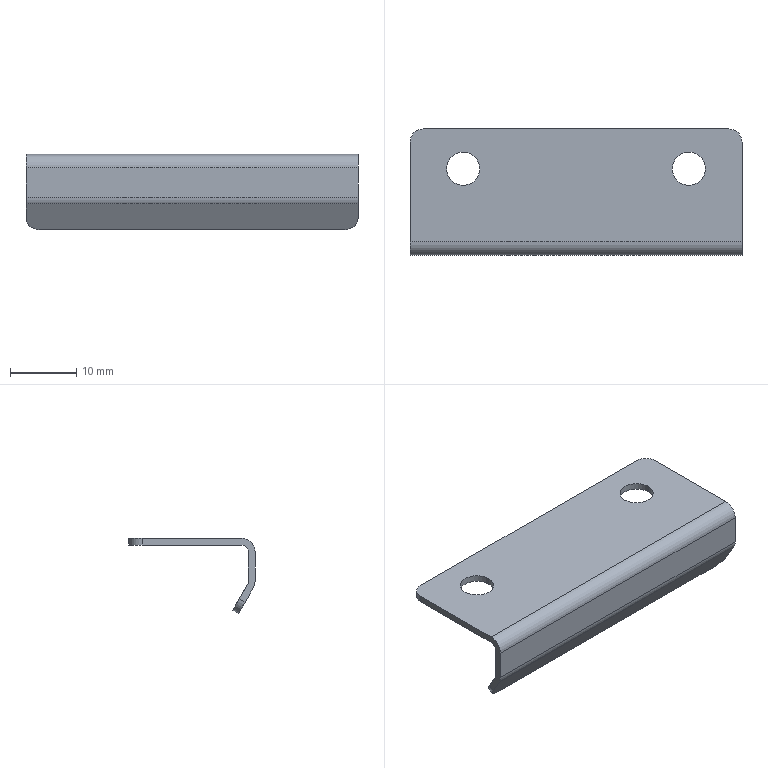Part | NX | features BREP 1 | 1 solid | 22 faces | box 50 x 19 x 11.33 mm | volume 1411 mm3 | cylinder 12 | plane 10 | commonest cylinder face diameters 4 x6 5 x4 2 x2
STEP:
#1=CARTESIAN_POINT('',(-14.5,3.5,1.));
#2=VERTEX_POINT('',#1);
#3=CARTESIAN_POINT('',(-19.5,3.5,1.));
#4=VERTEX_POINT('',#3);
#5=CARTESIAN_POINT('',(-17.,3.5,1.));
#6=DIRECTION('',(0.,0.,-1.));
#7=DIRECTION('',(-1.,0.,0.));
#8=AXIS2_PLACEMENT_3D('',#5,#6,#7);
#9=CIRCLE('',#8,2.5);
#10=EDGE_CURVE('',#2,#4,#9,.T.);
#11=ORIENTED_EDGE('',*,*,#10,.F.);
#12=CARTESIAN_POINT('',(-14.5,3.5,0.));
#13=VERTEX_POINT('',#12);
#14=CARTESIAN_POINT('',(-14.5,3.5,1.));
#15=DIRECTION('',(0.,0.,-1.));
#16=VECTOR('',#15,1000.);
#17=LINE('',#14,#16);
#18=EDGE_CURVE('',#2,#13,#17,.T.);
#19=ORIENTED_EDGE('',*,*,#18,.T.);
#20=CARTESIAN_POINT('',(-19.5,3.5,0.));
#21=VERTEX_POINT('',#20);
#22=CARTESIAN_POINT('',(-17.,3.5,0.));
#23=DIRECTION('',(0.,0.,-1.));
#24=DIRECTION('',(-1.,0.,0.));
#25=AXIS2_PLACEMENT_3D('',#22,#23,#24);
#26=CIRCLE('',#25,2.5);
#27=EDGE_CURVE('',#13,#21,#26,.T.);
#28=ORIENTED_EDGE('',*,*,#27,.T.);
#29=CARTESIAN_POINT('',(-19.5,3.5,1.));
#30=DIRECTION('',(0.,0.,-1.));
#31=VECTOR('',#30,1000.);
#32=LINE('',#29,#31);
#33=EDGE_CURVE('',#4,#21,#32,.T.);
#34=ORIENTED_EDGE('',*,*,#33,.F.);
#35=EDGE_LOOP('',(#11,#19,#28,#34));
#36=FACE_BOUND('',#35,.T.);
#37=CARTESIAN_POINT('',(-17.,3.5,1.));
#38=DIRECTION('',(0.,0.,-1.));
#39=DIRECTION('',(-1.,0.,0.));
#40=AXIS2_PLACEMENT_3D('',#37,#38,#39);
#41=CYLINDRICAL_SURFACE('',#40,2.5);
#42=ADVANCED_FACE('',(#36),#41,.F.);
#43=CARTESIAN_POINT('',(19.5,3.5,1.));
#44=VERTEX_POINT('',#43);
#45=CARTESIAN_POINT('',(14.5,3.5,1.));
#46=VERTEX_POINT('',#45);
#47=CARTESIAN_POINT('',(17.,3.5,1.));
#48=DIRECTION('',(0.,0.,-1.));
#49=DIRECTION('',(-1.,0.,0.));
#50=AXIS2_PLACEMENT_3D('',#47,#48,#49);
#51=CIRCLE('',#50,2.5);
#52=EDGE_CURVE('',#44,#46,#51,.T.);
#53=ORIENTED_EDGE('',*,*,#52,.F.);
#54=CARTESIAN_POINT('',(19.5,3.5,0.));
#55=VERTEX_POINT('',#54);
#56=CARTESIAN_POINT('',(19.5,3.5,1.));
#57=DIRECTION('',(0.,0.,-1.));
#58=VECTOR('',#57,1000.);
#59=LINE('',#56,#58);
#60=EDGE_CURVE('',#44,#55,#59,.T.);
#61=ORIENTED_EDGE('',*,*,#60,.T.);
#62=CARTESIAN_POINT('',(14.5,3.5,0.));
#63=VERTEX_POINT('',#62);
#64=CARTESIAN_POINT('',(17.,3.5,0.));
#65=DIRECTION('',(0.,0.,-1.));
#66=DIRECTION('',(-1.,0.,0.));
#67=AXIS2_PLACEMENT_3D('',#64,#65,#66);
#68=CIRCLE('',#67,2.5);
#69=EDGE_CURVE('',#55,#63,#68,.T.);
#70=ORIENTED_EDGE('',*,*,#69,.T.);
#71=CARTESIAN_POINT('',(14.5,3.5,1.));
#72=DIRECTION('',(0.,0.,-1.));
#73=VECTOR('',#72,1000.);
#74=LINE('',#71,#73);
#75=EDGE_CURVE('',#46,#63,#74,.T.);
#76=ORIENTED_EDGE('',*,*,#75,.F.);
#77=EDGE_LOOP('',(#53,#61,#70,#76));
#78=FACE_BOUND('',#77,.T.);
#79=CARTESIAN_POINT('',(17.,3.5,1.));
#80=DIRECTION('',(0.,0.,-1.));
#81=DIRECTION('',(-1.,0.,0.));
#82=AXIS2_PLACEMENT_3D('',#79,#80,#81);
#83=CYLINDRICAL_SURFACE('',#82,2.5);
#84=ADVANCED_FACE('',(#78),#83,.F.);
#85=CARTESIAN_POINT('',(25.,-7.5,0.));
#86=VERTEX_POINT('',#85);
#87=CARTESIAN_POINT('',(25.,7.5,0.));
#88=VERTEX_POINT('',#87);
#89=CARTESIAN_POINT('',(25.,-9.5,0.));
#90=DIRECTION('',(0.,1.,0.));
#91=VECTOR('',#90,1000.);
#92=LINE('',#89,#91);
#93=EDGE_CURVE('',#86,#88,#92,.T.);
#94=ORIENTED_EDGE('',*,*,#93,.T.);
#95=CARTESIAN_POINT('',(25.,7.5,1.));
#96=VERTEX_POINT('',#95);
#97=CARTESIAN_POINT('',(25.,7.5,1.));
#98=DIRECTION('',(0.,0.,1.));
#99=VECTOR('',#98,1000.);
#100=LINE('',#97,#99);
#101=EDGE_CURVE('',#88,#96,#100,.T.);
#102=ORIENTED_EDGE('',*,*,#101,.T.);
#103=CARTESIAN_POINT('',(25.,-7.5,1.));
#104=VERTEX_POINT('',#103);
#105=CARTESIAN_POINT('',(25.,-9.5,1.));
#106=DIRECTION('',(0.,1.,0.));
#107=VECTOR('',#106,1000.);
#108=LINE('',#105,#107);
#109=EDGE_CURVE('',#104,#96,#108,.T.);
#110=ORIENTED_EDGE('',*,*,#109,.F.);
#111=CARTESIAN_POINT('',(25.,-9.5,-1.));
#112=VERTEX_POINT('',#111);
#113=CARTESIAN_POINT('',(25.,-7.5,-1.));
#114=DIRECTION('',(1.,0.,0.));
#115=DIRECTION('',(0.,0.,1.));
#116=AXIS2_PLACEMENT_3D('',#113,#114,#115);
#117=CIRCLE('',#116,2.);
#118=EDGE_CURVE('',#104,#112,#117,.T.);
#119=ORIENTED_EDGE('',*,*,#118,.T.);
#120=CARTESIAN_POINT('',(25.,-9.5,-5.464));
#121=VERTEX_POINT('',#120);
#122=CARTESIAN_POINT('',(25.,-9.5,1.));
#123=DIRECTION('',(0.,0.,-1.));
#124=VECTOR('',#123,1000.);
#125=LINE('',#122,#124);
#126=EDGE_CURVE('',#112,#121,#125,.T.);
#127=ORIENTED_EDGE('',*,*,#126,.T.);
#128=CARTESIAN_POINT('',(25.,-9.232,-6.464));
#129=VERTEX_POINT('',#128);
#130=CARTESIAN_POINT('',(25.,-7.5,-5.464));
#131=DIRECTION('',(1.,0.,0.));
#132=DIRECTION('',(0.,0.,1.));
#133=AXIS2_PLACEMENT_3D('',#130,#131,#132);
#134=CIRCLE('',#133,2.);
#135=EDGE_CURVE('',#121,#129,#134,.T.);
#136=ORIENTED_EDGE('',*,*,#135,.T.);
#137=CARTESIAN_POINT('',(25.,-8.,-8.598));
#138=VERTEX_POINT('',#137);
#139=CARTESIAN_POINT('',(25.,-9.5,-6.));
#140=DIRECTION('',(0.,0.5,-0.866));
#141=VECTOR('',#140,1000.);
#142=LINE('',#139,#141);
#143=EDGE_CURVE('',#129,#138,#142,.T.);
#144=ORIENTED_EDGE('',*,*,#143,.T.);
#145=CARTESIAN_POINT('',(25.,-7.134,-8.098));
#146=VERTEX_POINT('',#145);
#147=CARTESIAN_POINT('',(25.,-7.134,-8.098));
#148=DIRECTION('',(0.,0.866,0.5));
#149=VECTOR('',#148,1000.);
#150=LINE('',#147,#149);
#151=EDGE_CURVE('',#138,#146,#150,.T.);
#152=ORIENTED_EDGE('',*,*,#151,.T.);
#153=CARTESIAN_POINT('',(25.,-8.366,-5.964));
#154=VERTEX_POINT('',#153);
#155=CARTESIAN_POINT('',(25.,-8.634,-5.5));
#156=DIRECTION('',(0.,-0.5,0.866));
#157=VECTOR('',#156,1000.);
#158=LINE('',#155,#157);
#159=EDGE_CURVE('',#146,#154,#158,.T.);
#160=ORIENTED_EDGE('',*,*,#159,.T.);
#161=CARTESIAN_POINT('',(25.,-8.5,-5.464));
#162=VERTEX_POINT('',#161);
#163=CARTESIAN_POINT('',(25.,-7.5,-5.464));
#164=DIRECTION('',(-1.,0.,0.));
#165=DIRECTION('',(0.,0.,1.));
#166=AXIS2_PLACEMENT_3D('',#163,#164,#165);
#167=CIRCLE('',#166,1.);
#168=EDGE_CURVE('',#154,#162,#167,.T.);
#169=ORIENTED_EDGE('',*,*,#168,.T.);
#170=CARTESIAN_POINT('',(25.,-8.5,-1.));
#171=VERTEX_POINT('',#170);
#172=CARTESIAN_POINT('',(25.,-8.5,-6.));
#173=DIRECTION('',(0.,0.,1.));
#174=VECTOR('',#173,1000.);
#175=LINE('',#172,#174);
#176=EDGE_CURVE('',#162,#171,#175,.T.);
#177=ORIENTED_EDGE('',*,*,#176,.T.);
#178=CARTESIAN_POINT('',(25.,-7.5,-1.));
#179=DIRECTION('',(-1.,0.,0.));
#180=DIRECTION('',(0.,0.,1.));
#181=AXIS2_PLACEMENT_3D('',#178,#179,#180);
#182=CIRCLE('',#181,1.);
#183=EDGE_CURVE('',#171,#86,#182,.T.);
#184=ORIENTED_EDGE('',*,*,#183,.T.);
#185=EDGE_LOOP('',(#94,#102,#110,#119,#127,#136,#144,#152,#160,#169,#177,#184));
#186=FACE_BOUND('',#185,.T.);
#187=CARTESIAN_POINT('',(25.,-9.5,1.));
#188=DIRECTION('',(-1.,0.,0.));
#189=DIRECTION('',(0.,0.,1.));
#190=AXIS2_PLACEMENT_3D('',#187,#188,#189);
#191=PLANE('',#190);
#192=ADVANCED_FACE('',(#186),#191,.F.);
#193=CARTESIAN_POINT('',(23.,9.5,0.));
#194=VERTEX_POINT('',#193);
#195=CARTESIAN_POINT('',(-23.,9.5,0.));
#196=VERTEX_POINT('',#195);
#197=CARTESIAN_POINT('',(-25.,9.5,0.));
#198=DIRECTION('',(-1.,0.,0.));
#199=VECTOR('',#198,1000.);
#200=LINE('',#197,#199);
#201=EDGE_CURVE('',#194,#196,#200,.T.);
#202=ORIENTED_EDGE('',*,*,#201,.T.);
#203=CARTESIAN_POINT('',(-23.,9.5,1.));
#204=VERTEX_POINT('',#203);
#205=CARTESIAN_POINT('',(-23.,9.5,1.));
#206=DIRECTION('',(0.,0.,1.));
#207=VECTOR('',#206,1000.);
#208=LINE('',#205,#207);
#209=EDGE_CURVE('',#196,#204,#208,.T.);
#210=ORIENTED_EDGE('',*,*,#209,.T.);
#211=CARTESIAN_POINT('',(23.,9.5,1.));
#212=VERTEX_POINT('',#211);
#213=CARTESIAN_POINT('',(-25.,9.5,1.));
#214=DIRECTION('',(-1.,0.,0.));
#215=VECTOR('',#214,1000.);
#216=LINE('',#213,#215);
#217=EDGE_CURVE('',#212,#204,#216,.T.);
#218=ORIENTED_EDGE('',*,*,#217,.F.);
#219=CARTESIAN_POINT('',(23.,9.5,1.));
#220=DIRECTION('',(0.,0.,-1.));
#221=VECTOR('',#220,1000.);
#222=LINE('',#219,#221);
#223=EDGE_CURVE('',#212,#194,#222,.T.);
#224=ORIENTED_EDGE('',*,*,#223,.T.);
#225=EDGE_LOOP('',(#202,#210,#218,#224));
#226=FACE_BOUND('',#225,.T.);
#227=CARTESIAN_POINT('',(-25.,9.5,1.));
#228=DIRECTION('',(0.,-1.,0.));
#229=DIRECTION('',(0.,0.,-1.));
#230=AXIS2_PLACEMENT_3D('',#227,#228,#229);
#231=PLANE('',#230);
#232=ADVANCED_FACE('',(#226),#231,.F.);
#233=CARTESIAN_POINT('',(-25.,7.5,1.));
#234=VERTEX_POINT('',#233);
#235=CARTESIAN_POINT('',(-25.,-7.5,1.));
#236=VERTEX_POINT('',#235);
#237=CARTESIAN_POINT('',(-25.,-9.5,1.));
#238=DIRECTION('',(0.,-1.,0.));
#239=VECTOR('',#238,1000.);
#240=LINE('',#237,#239);
#241=EDGE_CURVE('',#234,#236,#240,.T.);
#242=ORIENTED_EDGE('',*,*,#241,.F.);
#243=CARTESIAN_POINT('',(-25.,7.5,0.));
#244=VERTEX_POINT('',#243);
#245=CARTESIAN_POINT('',(-25.,7.5,1.));
#246=DIRECTION('',(0.,0.,-1.));
#247=VECTOR('',#246,1000.);
#248=LINE('',#245,#247);
#249=EDGE_CURVE('',#234,#244,#248,.T.);
#250=ORIENTED_EDGE('',*,*,#249,.T.);
#251=CARTESIAN_POINT('',(-25.,-7.5,0.));
#252=VERTEX_POINT('',#251);
#253=CARTESIAN_POINT('',(-25.,-9.5,0.));
#254=DIRECTION('',(0.,-1.,0.));
#255=VECTOR('',#254,1000.);
#256=LINE('',#253,#255);
#257=EDGE_CURVE('',#244,#252,#256,.T.);
#258=ORIENTED_EDGE('',*,*,#257,.T.);
#259=CARTESIAN_POINT('',(-25.,-8.5,-1.));
#260=VERTEX_POINT('',#259);
#261=CARTESIAN_POINT('',(-25.,-7.5,-1.));
#262=DIRECTION('',(1.,0.,0.));
#263=DIRECTION('',(0.,0.,-1.));
#264=AXIS2_PLACEMENT_3D('',#261,#262,#263);
#265=CIRCLE('',#264,1.);
#266=EDGE_CURVE('',#252,#260,#265,.T.);
#267=ORIENTED_EDGE('',*,*,#266,.T.);
#268=CARTESIAN_POINT('',(-25.,-8.5,-5.464));
#269=VERTEX_POINT('',#268);
#270=CARTESIAN_POINT('',(-25.,-8.5,-6.));
#271=DIRECTION('',(0.,0.,1.));
#272=VECTOR('',#271,1000.);
#273=LINE('',#270,#272);
#274=EDGE_CURVE('',#269,#260,#273,.T.);
#275=ORIENTED_EDGE('',*,*,#274,.F.);
#276=CARTESIAN_POINT('',(-25.,-8.366,-5.964));
#277=VERTEX_POINT('',#276);
#278=CARTESIAN_POINT('',(-25.,-7.5,-5.464));
#279=DIRECTION('',(1.,0.,0.));
#280=DIRECTION('',(0.,0.,-1.));
#281=AXIS2_PLACEMENT_3D('',#278,#279,#280);
#282=CIRCLE('',#281,1.);
#283=EDGE_CURVE('',#269,#277,#282,.T.);
#284=ORIENTED_EDGE('',*,*,#283,.T.);
#285=CARTESIAN_POINT('',(-25.,-7.134,-8.098));
#286=VERTEX_POINT('',#285);
#287=CARTESIAN_POINT('',(-25.,-8.634,-5.5));
#288=DIRECTION('',(0.,0.5,-0.866));
#289=VECTOR('',#288,1000.);
#290=LINE('',#287,#289);
#291=EDGE_CURVE('',#277,#286,#290,.T.);
#292=ORIENTED_EDGE('',*,*,#291,.T.);
#293=CARTESIAN_POINT('',(-25.,-8.,-8.598));
#294=VERTEX_POINT('',#293);
#295=CARTESIAN_POINT('',(-25.,-8.,-8.598));
#296=DIRECTION('',(0.,-0.866,-0.5));
#297=VECTOR('',#296,1000.);
#298=LINE('',#295,#297);
#299=EDGE_CURVE('',#286,#294,#298,.T.);
#300=ORIENTED_EDGE('',*,*,#299,.T.);
#301=CARTESIAN_POINT('',(-25.,-9.232,-6.464));
#302=VERTEX_POINT('',#301);
#303=CARTESIAN_POINT('',(-25.,-9.5,-6.));
#304=DIRECTION('',(0.,-0.5,0.866));
#305=VECTOR('',#304,1000.);
#306=LINE('',#303,#305);
#307=EDGE_CURVE('',#294,#302,#306,.T.);
#308=ORIENTED_EDGE('',*,*,#307,.T.);
#309=CARTESIAN_POINT('',(-25.,-9.5,-5.464));
#310=VERTEX_POINT('',#309);
#311=CARTESIAN_POINT('',(-25.,-7.5,-5.464));
#312=DIRECTION('',(-1.,0.,0.));
#313=DIRECTION('',(0.,0.,-1.));
#314=AXIS2_PLACEMENT_3D('',#311,#312,#313);
#315=CIRCLE('',#314,2.);
#316=EDGE_CURVE('',#302,#310,#315,.T.);
#317=ORIENTED_EDGE('',*,*,#316,.T.);
#318=CARTESIAN_POINT('',(-25.,-9.5,-1.));
#319=VERTEX_POINT('',#318);
#320=CARTESIAN_POINT('',(-25.,-9.5,1.));
#321=DIRECTION('',(0.,0.,-1.));
#322=VECTOR('',#321,1000.);
#323=LINE('',#320,#322);
#324=EDGE_CURVE('',#319,#310,#323,.T.);
#325=ORIENTED_EDGE('',*,*,#324,.F.);
#326=CARTESIAN_POINT('',(-25.,-7.5,-1.));
#327=DIRECTION('',(-1.,0.,0.));
#328=DIRECTION('',(0.,0.,-1.));
#329=AXIS2_PLACEMENT_3D('',#326,#327,#328);
#330=CIRCLE('',#329,2.);
#331=EDGE_CURVE('',#319,#236,#330,.T.);
#332=ORIENTED_EDGE('',*,*,#331,.T.);
#333=EDGE_LOOP('',(#242,#250,#258,#267,#275,#284,#292,#300,#308,#317,#325,#332));
#334=FACE_BOUND('',#333,.T.);
#335=CARTESIAN_POINT('',(-25.,-9.5,1.));
#336=DIRECTION('',(1.,0.,0.));
#337=DIRECTION('',(0.,1.,0.));
#338=AXIS2_PLACEMENT_3D('',#335,#336,#337);
#339=PLANE('',#338);
#340=ADVANCED_FACE('',(#334),#339,.F.);
#341=ORIENTED_EDGE('',*,*,#324,.T.);
#342=CARTESIAN_POINT('',(25.,-9.5,-5.464));
#343=DIRECTION('',(1.,0.,0.));
#344=VECTOR('',#343,1000.);
#345=LINE('',#342,#344);
#346=EDGE_CURVE('',#310,#121,#345,.T.);
#347=ORIENTED_EDGE('',*,*,#346,.T.);
#348=ORIENTED_EDGE('',*,*,#126,.F.);
#349=CARTESIAN_POINT('',(-25.,-9.5,-1.));
#350=DIRECTION('',(-1.,0.,0.));
#351=VECTOR('',#350,1000.);
#352=LINE('',#349,#351);
#353=EDGE_CURVE('',#112,#319,#352,.T.);
#354=ORIENTED_EDGE('',*,*,#353,.T.);
#355=EDGE_LOOP('',(#341,#347,#348,#354));
#356=FACE_BOUND('',#355,.T.);
#357=CARTESIAN_POINT('',(-25.,-9.5,1.));
#358=DIRECTION('',(0.,1.,0.));
#359=DIRECTION('',(1.,0.,0.));
#360=AXIS2_PLACEMENT_3D('',#357,#358,#359);
#361=PLANE('',#360);
#362=ADVANCED_FACE('',(#356),#361,.F.);
#363=ORIENTED_EDGE('',*,*,#217,.T.);
#364=CARTESIAN_POINT('',(-23.,7.5,1.));
#365=DIRECTION('',(0.,0.,1.));
#366=DIRECTION('',(-1.,0.,0.));
#367=AXIS2_PLACEMENT_3D('',#364,#365,#366);
#368=CIRCLE('',#367,2.);
#369=EDGE_CURVE('',#204,#234,#368,.T.);
#370=ORIENTED_EDGE('',*,*,#369,.T.);
#371=ORIENTED_EDGE('',*,*,#241,.T.);
#372=CARTESIAN_POINT('',(0.,-7.5,1.));
#373=DIRECTION('',(1.,0.,0.));
#374=VECTOR('',#373,1000.);
#375=LINE('',#372,#374);
#376=EDGE_CURVE('',#236,#104,#375,.T.);
#377=ORIENTED_EDGE('',*,*,#376,.T.);
#378=ORIENTED_EDGE('',*,*,#109,.T.);
#379=CARTESIAN_POINT('',(23.,7.5,1.));
#380=DIRECTION('',(0.,0.,1.));
#381=DIRECTION('',(-1.,0.,0.));
#382=AXIS2_PLACEMENT_3D('',#379,#380,#381);
#383=CIRCLE('',#382,2.);
#384=EDGE_CURVE('',#96,#212,#383,.T.);
#385=ORIENTED_EDGE('',*,*,#384,.T.);
#386=EDGE_LOOP('',(#363,#370,#371,#377,#378,#385));
#387=FACE_BOUND('',#386,.T.);
#388=CARTESIAN_POINT('',(-17.,3.5,1.));
#389=DIRECTION('',(0.,0.,-1.));
#390=DIRECTION('',(-1.,0.,0.));
#391=AXIS2_PLACEMENT_3D('',#388,#389,#390);
#392=CIRCLE('',#391,2.5);
#393=EDGE_CURVE('',#4,#2,#392,.T.);
#394=ORIENTED_EDGE('',*,*,#393,.T.);
#395=ORIENTED_EDGE('',*,*,#10,.T.);
#396=EDGE_LOOP('',(#394,#395));
#397=FACE_BOUND('',#396,.T.);
#398=CARTESIAN_POINT('',(17.,3.5,1.));
#399=DIRECTION('',(0.,0.,-1.));
#400=DIRECTION('',(-1.,0.,0.));
#401=AXIS2_PLACEMENT_3D('',#398,#399,#400);
#402=CIRCLE('',#401,2.5);
#403=EDGE_CURVE('',#46,#44,#402,.T.);
#404=ORIENTED_EDGE('',*,*,#403,.T.);
#405=ORIENTED_EDGE('',*,*,#52,.T.);
#406=EDGE_LOOP('',(#404,#405));
#407=FACE_BOUND('',#406,.T.);
#408=CARTESIAN_POINT('',(0.,0.,1.));
#409=DIRECTION('',(0.,0.,-1.));
#410=DIRECTION('',(0.,-1.,0.));
#411=AXIS2_PLACEMENT_3D('',#408,#409,#410);
#412=PLANE('',#411);
#413=ADVANCED_FACE('',(#387,#397,#407),#412,.F.);
#414=ORIENTED_EDGE('',*,*,#257,.F.);
#415=CARTESIAN_POINT('',(-23.,7.5,0.));
#416=DIRECTION('',(0.,0.,-1.));
#417=DIRECTION('',(-1.,0.,0.));
#418=AXIS2_PLACEMENT_3D('',#415,#416,#417);
#419=CIRCLE('',#418,2.);
#420=EDGE_CURVE('',#244,#196,#419,.T.);
#421=ORIENTED_EDGE('',*,*,#420,.T.);
#422=ORIENTED_EDGE('',*,*,#201,.F.);
#423=CARTESIAN_POINT('',(23.,7.5,0.));
#424=DIRECTION('',(0.,0.,-1.));
#425=DIRECTION('',(-1.,0.,0.));
#426=AXIS2_PLACEMENT_3D('',#423,#424,#425);
#427=CIRCLE('',#426,2.);
#428=EDGE_CURVE('',#194,#88,#427,.T.);
#429=ORIENTED_EDGE('',*,*,#428,.T.);
#430=ORIENTED_EDGE('',*,*,#93,.F.);
#431=CARTESIAN_POINT('',(0.,-7.5,0.));
#432=DIRECTION('',(-1.,0.,0.));
#433=VECTOR('',#432,1000.);
#434=LINE('',#431,#433);
#435=EDGE_CURVE('',#86,#252,#434,.T.);
#436=ORIENTED_EDGE('',*,*,#435,.T.);
#437=EDGE_LOOP('',(#414,#421,#422,#429,#430,#436));
#438=FACE_BOUND('',#437,.T.);
#439=CARTESIAN_POINT('',(-17.,3.5,0.));
#440=DIRECTION('',(0.,0.,-1.));
#441=DIRECTION('',(-1.,0.,0.));
#442=AXIS2_PLACEMENT_3D('',#439,#440,#441);
#443=CIRCLE('',#442,2.5);
#444=EDGE_CURVE('',#21,#13,#443,.T.);
#445=ORIENTED_EDGE('',*,*,#444,.F.);
#446=ORIENTED_EDGE('',*,*,#27,.F.);
#447=EDGE_LOOP('',(#445,#446));
#448=FACE_BOUND('',#447,.T.);
#449=CARTESIAN_POINT('',(17.,3.5,0.));
#450=DIRECTION('',(0.,0.,-1.));
#451=DIRECTION('',(-1.,0.,0.));
#452=AXIS2_PLACEMENT_3D('',#449,#450,#451);
#453=CIRCLE('',#452,2.5);
#454=EDGE_CURVE('',#63,#55,#453,.T.);
#455=ORIENTED_EDGE('',*,*,#454,.F.);
#456=ORIENTED_EDGE('',*,*,#69,.F.);
#457=EDGE_LOOP('',(#455,#456));
#458=FACE_BOUND('',#457,.T.);
#459=CARTESIAN_POINT('',(0.,0.,0.));
#460=DIRECTION('',(0.,0.,-1.));
#461=DIRECTION('',(0.,-1.,0.));
#462=AXIS2_PLACEMENT_3D('',#459,#460,#461);
#463=PLANE('',#462);
#464=ADVANCED_FACE('',(#438,#448,#458),#463,.T.);
#465=ORIENTED_EDGE('',*,*,#176,.F.);
#466=CARTESIAN_POINT('',(-25.,-8.5,-5.464));
#467=DIRECTION('',(-1.,0.,0.));
#468=VECTOR('',#467,1000.);
#469=LINE('',#466,#468);
#470=EDGE_CURVE('',#162,#269,#469,.T.);
#471=ORIENTED_EDGE('',*,*,#470,.T.);
#472=ORIENTED_EDGE('',*,*,#274,.T.);
#473=CARTESIAN_POINT('',(-25.,-8.5,-1.));
#474=DIRECTION('',(1.,0.,0.));
#475=VECTOR('',#474,1000.);
#476=LINE('',#473,#475);
#477=EDGE_CURVE('',#260,#171,#476,.T.);
#478=ORIENTED_EDGE('',*,*,#477,.T.);
#479=EDGE_LOOP('',(#465,#471,#472,#478));
#480=FACE_BOUND('',#479,.T.);
#481=CARTESIAN_POINT('',(-25.,-8.5,-6.));
#482=DIRECTION('',(0.,-1.,0.));
#483=DIRECTION('',(-1.,0.,0.));
#484=AXIS2_PLACEMENT_3D('',#481,#482,#483);
#485=PLANE('',#484);
#486=ADVANCED_FACE('',(#480),#485,.F.);
#487=CARTESIAN_POINT('',(23.,-6.134,-9.83));
#488=VERTEX_POINT('',#487);
#489=CARTESIAN_POINT('',(-23.,-6.134,-9.83));
#490=VERTEX_POINT('',#489);
#491=CARTESIAN_POINT('',(30.887,-6.134,-9.83));
#492=DIRECTION('',(-1.,0.,0.));
#493=VECTOR('',#492,1000.);
#494=LINE('',#491,#493);
#495=EDGE_CURVE('',#488,#490,#494,.T.);
#496=ORIENTED_EDGE('',*,*,#495,.T.);
#497=CARTESIAN_POINT('',(-23.,-7.134,-8.098));
#498=DIRECTION('',(0.,0.866,0.5));
#499=DIRECTION('',(0.,-0.5,0.866));
#500=AXIS2_PLACEMENT_3D('',#497,#498,#499);
#501=CIRCLE('',#500,2.);
#502=EDGE_CURVE('',#490,#286,#501,.T.);
#503=ORIENTED_EDGE('',*,*,#502,.T.);
#504=ORIENTED_EDGE('',*,*,#291,.F.);
#505=CARTESIAN_POINT('',(30.887,-8.366,-5.964));
#506=DIRECTION('',(1.,0.,0.));
#507=VECTOR('',#506,1000.);
#508=LINE('',#505,#507);
#509=EDGE_CURVE('',#277,#154,#508,.T.);
#510=ORIENTED_EDGE('',*,*,#509,.T.);
#511=ORIENTED_EDGE('',*,*,#159,.F.);
#512=CARTESIAN_POINT('',(23.,-7.134,-8.098));
#513=DIRECTION('',(0.,0.866,0.5));
#514=DIRECTION('',(0.,-0.5,0.866));
#515=AXIS2_PLACEMENT_3D('',#512,#513,#514);
#516=CIRCLE('',#515,2.);
#517=EDGE_CURVE('',#146,#488,#516,.T.);
#518=ORIENTED_EDGE('',*,*,#517,.T.);
#519=EDGE_LOOP('',(#496,#503,#504,#510,#511,#518));
#520=FACE_BOUND('',#519,.T.);
#521=CARTESIAN_POINT('',(30.887,-8.634,-5.5));
#522=DIRECTION('',(0.,0.866,0.5));
#523=DIRECTION('',(1.,0.,0.));
#524=AXIS2_PLACEMENT_3D('',#521,#522,#523);
#525=PLANE('',#524);
#526=ADVANCED_FACE('',(#520),#525,.T.);
#527=ORIENTED_EDGE('',*,*,#307,.F.);
#528=CARTESIAN_POINT('',(-23.,-7.,-10.33));
#529=VERTEX_POINT('',#528);
#530=CARTESIAN_POINT('',(-23.,-8.,-8.598));
#531=DIRECTION('',(0.,-0.866,-0.5));
#532=DIRECTION('',(0.,0.5,-0.866));
#533=AXIS2_PLACEMENT_3D('',#530,#531,#532);
#534=CIRCLE('',#533,2.);
#535=EDGE_CURVE('',#294,#529,#534,.T.);
#536=ORIENTED_EDGE('',*,*,#535,.T.);
#537=CARTESIAN_POINT('',(23.,-7.,-10.33));
#538=VERTEX_POINT('',#537);
#539=CARTESIAN_POINT('',(30.887,-7.,-10.33));
#540=DIRECTION('',(-1.,0.,0.));
#541=VECTOR('',#540,1000.);
#542=LINE('',#539,#541);
#543=EDGE_CURVE('',#538,#529,#542,.T.);
#544=ORIENTED_EDGE('',*,*,#543,.F.);
#545=CARTESIAN_POINT('',(23.,-8.,-8.598));
#546=DIRECTION('',(0.,-0.866,-0.5));
#547=DIRECTION('',(0.,0.5,-0.866));
#548=AXIS2_PLACEMENT_3D('',#545,#546,#547);
#549=CIRCLE('',#548,2.);
#550=EDGE_CURVE('',#538,#138,#549,.T.);
#551=ORIENTED_EDGE('',*,*,#550,.T.);
#552=ORIENTED_EDGE('',*,*,#143,.F.);
#553=CARTESIAN_POINT('',(-25.,-9.232,-6.464));
#554=DIRECTION('',(-1.,0.,0.));
#555=VECTOR('',#554,1000.);
#556=LINE('',#553,#555);
#557=EDGE_CURVE('',#129,#302,#556,.T.);
#558=ORIENTED_EDGE('',*,*,#557,.T.);
#559=EDGE_LOOP('',(#527,#536,#544,#551,#552,#558));
#560=FACE_BOUND('',#559,.T.);
#561=CARTESIAN_POINT('',(30.887,-9.5,-6.));
#562=DIRECTION('',(0.,-0.866,-0.5));
#563=DIRECTION('',(0.,0.5,-0.866));
#564=AXIS2_PLACEMENT_3D('',#561,#562,#563);
#565=PLANE('',#564);
#566=ADVANCED_FACE('',(#560),#565,.T.);
#567=ORIENTED_EDGE('',*,*,#543,.T.);
#568=CARTESIAN_POINT('',(-23.,-6.134,-9.83));
#569=DIRECTION('',(0.,0.866,0.5));
#570=VECTOR('',#569,1000.);
#571=LINE('',#568,#570);
#572=EDGE_CURVE('',#529,#490,#571,.T.);
#573=ORIENTED_EDGE('',*,*,#572,.T.);
#574=ORIENTED_EDGE('',*,*,#495,.F.);
#575=CARTESIAN_POINT('',(23.,-7.,-10.33));
#576=DIRECTION('',(0.,-0.866,-0.5));
#577=VECTOR('',#576,1000.);
#578=LINE('',#575,#577);
#579=EDGE_CURVE('',#488,#538,#578,.T.);
#580=ORIENTED_EDGE('',*,*,#579,.T.);
#581=EDGE_LOOP('',(#567,#573,#574,#580));
#582=FACE_BOUND('',#581,.T.);
#583=CARTESIAN_POINT('',(30.887,-6.134,-9.83));
#584=DIRECTION('',(0.,0.5,-0.866));
#585=DIRECTION('',(-1.,0.,0.));
#586=AXIS2_PLACEMENT_3D('',#583,#584,#585);
#587=PLANE('',#586);
#588=ADVANCED_FACE('',(#582),#587,.T.);
#589=ORIENTED_EDGE('',*,*,#168,.F.);
#590=ORIENTED_EDGE('',*,*,#509,.F.);
#591=ORIENTED_EDGE('',*,*,#283,.F.);
#592=ORIENTED_EDGE('',*,*,#470,.F.);
#593=EDGE_LOOP('',(#589,#590,#591,#592));
#594=FACE_BOUND('',#593,.T.);
#595=CARTESIAN_POINT('',(-25.,-7.5,-5.464));
#596=DIRECTION('',(-1.,0.,0.));
#597=DIRECTION('',(0.,0.,1.));
#598=AXIS2_PLACEMENT_3D('',#595,#596,#597);
#599=CYLINDRICAL_SURFACE('',#598,1.);
#600=ADVANCED_FACE('',(#594),#599,.F.);
#601=ORIENTED_EDGE('',*,*,#266,.F.);
#602=ORIENTED_EDGE('',*,*,#435,.F.);
#603=ORIENTED_EDGE('',*,*,#183,.F.);
#604=ORIENTED_EDGE('',*,*,#477,.F.);
#605=EDGE_LOOP('',(#601,#602,#603,#604));
#606=FACE_BOUND('',#605,.T.);
#607=CARTESIAN_POINT('',(-25.,-7.5,-1.));
#608=DIRECTION('',(1.,0.,0.));
#609=DIRECTION('',(0.,1.,0.));
#610=AXIS2_PLACEMENT_3D('',#607,#608,#609);
#611=CYLINDRICAL_SURFACE('',#610,1.);
#612=ADVANCED_FACE('',(#606),#611,.F.);
#613=ORIENTED_EDGE('',*,*,#369,.F.);
#614=ORIENTED_EDGE('',*,*,#209,.F.);
#615=ORIENTED_EDGE('',*,*,#420,.F.);
#616=ORIENTED_EDGE('',*,*,#249,.F.);
#617=EDGE_LOOP('',(#613,#614,#615,#616));
#618=FACE_BOUND('',#617,.T.);
#619=CARTESIAN_POINT('',(-23.,7.5,1.));
#620=DIRECTION('',(0.,0.,-1.));
#621=DIRECTION('',(-1.,0.,0.));
#622=AXIS2_PLACEMENT_3D('',#619,#620,#621);
#623=CYLINDRICAL_SURFACE('',#622,2.);
#624=ADVANCED_FACE('',(#618),#623,.T.);
#625=ORIENTED_EDGE('',*,*,#384,.F.);
#626=ORIENTED_EDGE('',*,*,#101,.F.);
#627=ORIENTED_EDGE('',*,*,#428,.F.);
#628=ORIENTED_EDGE('',*,*,#223,.F.);
#629=EDGE_LOOP('',(#625,#626,#627,#628));
#630=FACE_BOUND('',#629,.T.);
#631=CARTESIAN_POINT('',(23.,7.5,1.));
#632=DIRECTION('',(0.,0.,-1.));
#633=DIRECTION('',(-1.,0.,0.));
#634=AXIS2_PLACEMENT_3D('',#631,#632,#633);
#635=CYLINDRICAL_SURFACE('',#634,2.);
#636=ADVANCED_FACE('',(#630),#635,.T.);
#637=ORIENTED_EDGE('',*,*,#502,.F.);
#638=ORIENTED_EDGE('',*,*,#572,.F.);
#639=ORIENTED_EDGE('',*,*,#535,.F.);
#640=ORIENTED_EDGE('',*,*,#299,.F.);
#641=EDGE_LOOP('',(#637,#638,#639,#640));
#642=FACE_BOUND('',#641,.T.);
#643=CARTESIAN_POINT('',(-23.,-4.969,-6.848));
#644=DIRECTION('',(0.,0.866,0.5));
#645=DIRECTION('',(0.,-0.5,0.866));
#646=AXIS2_PLACEMENT_3D('',#643,#644,#645);
#647=CYLINDRICAL_SURFACE('',#646,2.);
#648=ADVANCED_FACE('',(#642),#647,.T.);
#649=ORIENTED_EDGE('',*,*,#550,.F.);
#650=ORIENTED_EDGE('',*,*,#579,.F.);
#651=ORIENTED_EDGE('',*,*,#517,.F.);
#652=ORIENTED_EDGE('',*,*,#151,.F.);
#653=EDGE_LOOP('',(#649,#650,#651,#652));
#654=FACE_BOUND('',#653,.T.);
#655=CARTESIAN_POINT('',(23.,-4.969,-6.848));
#656=DIRECTION('',(0.,-0.866,-0.5));
#657=DIRECTION('',(0.,0.5,-0.866));
#658=AXIS2_PLACEMENT_3D('',#655,#656,#657);
#659=CYLINDRICAL_SURFACE('',#658,2.);
#660=ADVANCED_FACE('',(#654),#659,.T.);
#661=ORIENTED_EDGE('',*,*,#135,.F.);
#662=ORIENTED_EDGE('',*,*,#346,.F.);
#663=ORIENTED_EDGE('',*,*,#316,.F.);
#664=ORIENTED_EDGE('',*,*,#557,.F.);
#665=EDGE_LOOP('',(#661,#662,#663,#664));
#666=FACE_BOUND('',#665,.T.);
#667=CARTESIAN_POINT('',(30.887,-7.5,-5.464));
#668=DIRECTION('',(1.,0.,0.));
#669=DIRECTION('',(0.,0.,-1.));
#670=AXIS2_PLACEMENT_3D('',#667,#668,#669);
#671=CYLINDRICAL_SURFACE('',#670,2.);
#672=ADVANCED_FACE('',(#666),#671,.T.);
#673=ORIENTED_EDGE('',*,*,#331,.F.);
#674=ORIENTED_EDGE('',*,*,#353,.F.);
#675=ORIENTED_EDGE('',*,*,#118,.F.);
#676=ORIENTED_EDGE('',*,*,#376,.F.);
#677=EDGE_LOOP('',(#673,#674,#675,#676));
#678=FACE_BOUND('',#677,.T.);
#679=CARTESIAN_POINT('',(0.,-7.5,-1.));
#680=DIRECTION('',(1.,0.,0.));
#681=DIRECTION('',(0.,0.,-1.));
#682=AXIS2_PLACEMENT_3D('',#679,#680,#681);
#683=CYLINDRICAL_SURFACE('',#682,2.);
#684=ADVANCED_FACE('',(#678),#683,.T.);
#685=ORIENTED_EDGE('',*,*,#60,.F.);
#686=ORIENTED_EDGE('',*,*,#403,.F.);
#687=ORIENTED_EDGE('',*,*,#75,.T.);
#688=ORIENTED_EDGE('',*,*,#454,.T.);
#689=EDGE_LOOP('',(#685,#686,#687,#688));
#690=FACE_BOUND('',#689,.T.);
#691=CARTESIAN_POINT('',(17.,3.5,1.));
#692=DIRECTION('',(0.,0.,-1.));
#693=DIRECTION('',(-1.,0.,0.));
#694=AXIS2_PLACEMENT_3D('',#691,#692,#693);
#695=CYLINDRICAL_SURFACE('',#694,2.5);
#696=ADVANCED_FACE('',(#690),#695,.F.);
#697=ORIENTED_EDGE('',*,*,#18,.F.);
#698=ORIENTED_EDGE('',*,*,#393,.F.);
#699=ORIENTED_EDGE('',*,*,#33,.T.);
#700=ORIENTED_EDGE('',*,*,#444,.T.);
#701=EDGE_LOOP('',(#697,#698,#699,#700));
#702=FACE_BOUND('',#701,.T.);
#703=CARTESIAN_POINT('',(-17.,3.5,1.));
#704=DIRECTION('',(0.,0.,-1.));
#705=DIRECTION('',(-1.,0.,0.));
#706=AXIS2_PLACEMENT_3D('',#703,#704,#705);
#707=CYLINDRICAL_SURFACE('',#706,2.5);
#708=ADVANCED_FACE('',(#702),#707,.F.);
#709=CLOSED_SHELL('',(#42,#84,#192,#232,#340,#362,#413,#464,#486,#526,#566,#588,#600,#612,#624,#636,#648,#660,#672,#684,#696,#708));
#710=MANIFOLD_SOLID_BREP('',#709);
#711=(LENGTH_UNIT()NAMED_UNIT(*)SI_UNIT(.MILLI.,.METRE.));
#712=UNCERTAINTY_MEASURE_WITH_UNIT(LENGTH_MEASURE(0.00001),#711,'','');
#713=(NAMED_UNIT(*)PLANE_ANGLE_UNIT()SI_UNIT($,.RADIAN.));
#714=(NAMED_UNIT(*)SI_UNIT($,.STERADIAN.)SOLID_ANGLE_UNIT());
#715=(GEOMETRIC_REPRESENTATION_CONTEXT(3)GLOBAL_UNCERTAINTY_ASSIGNED_CONTEXT((#712))GLOBAL_UNIT_ASSIGNED_CONTEXT((#711,#713,#714))REPRESENTATION_CONTEXT('',''));
#716=ADVANCED_BREP_SHAPE_REPRESENTATION('',(#710),#715);